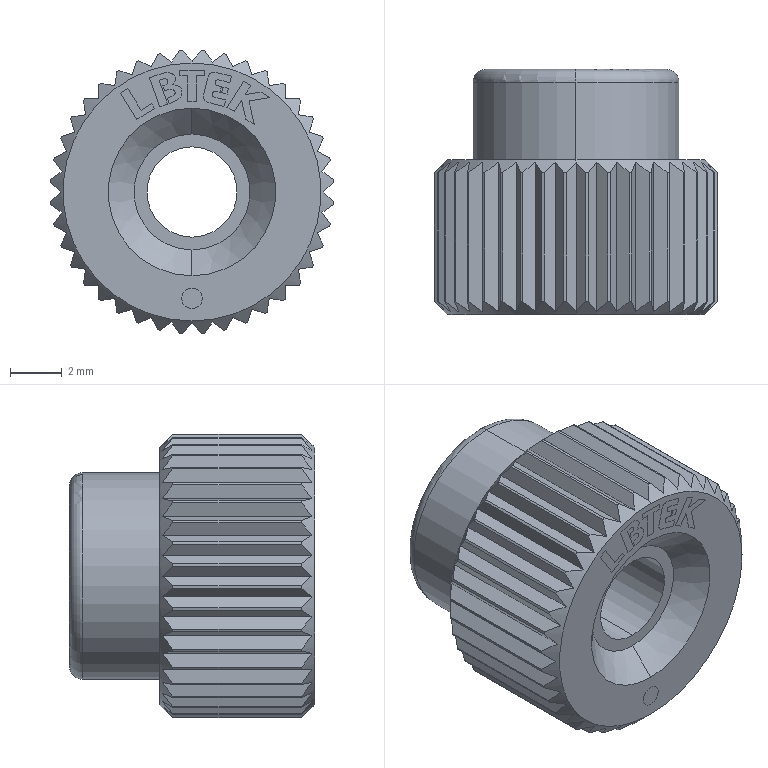Part | STEP file | 1 solid | 146 faces | box 10.973 x 9.5 x 10.973 mm | volume 552.638 mm3 | plane 92 | cylinder 46 | cone 6 | torus 2 | commonest cylinder face diameters 11 x40 3.5 x2 5 x2 8 x2